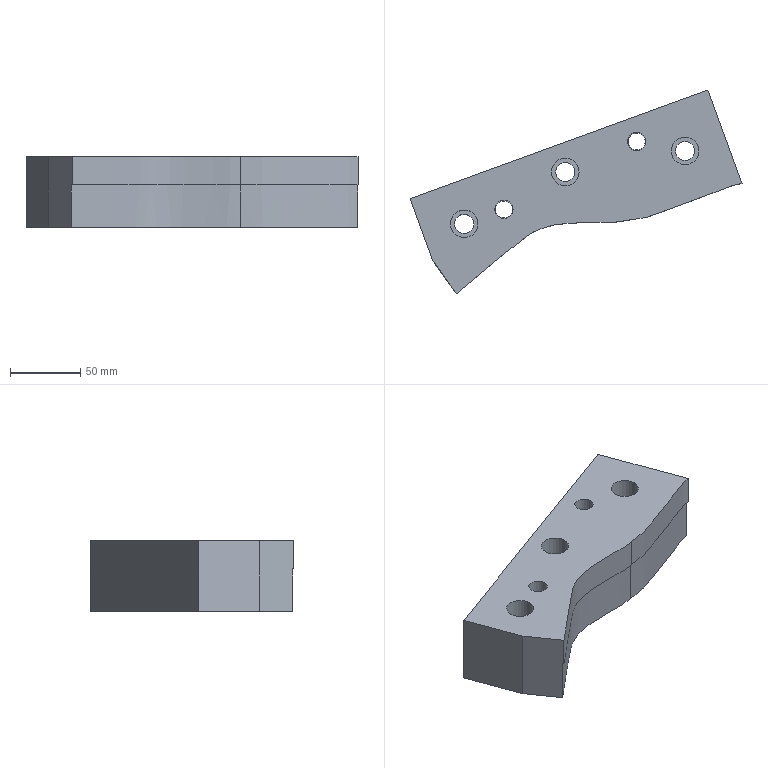Part | NX | features solid 2 | 1 solid | 26 faces | box 235.557 x 144.564 x 50 mm | volume 672239 mm3 | plane 12 | cylinder 10 | spline 4 | commonest cylinder face diameters 13.5 x3 19.5 x3 12 x2 13 x2